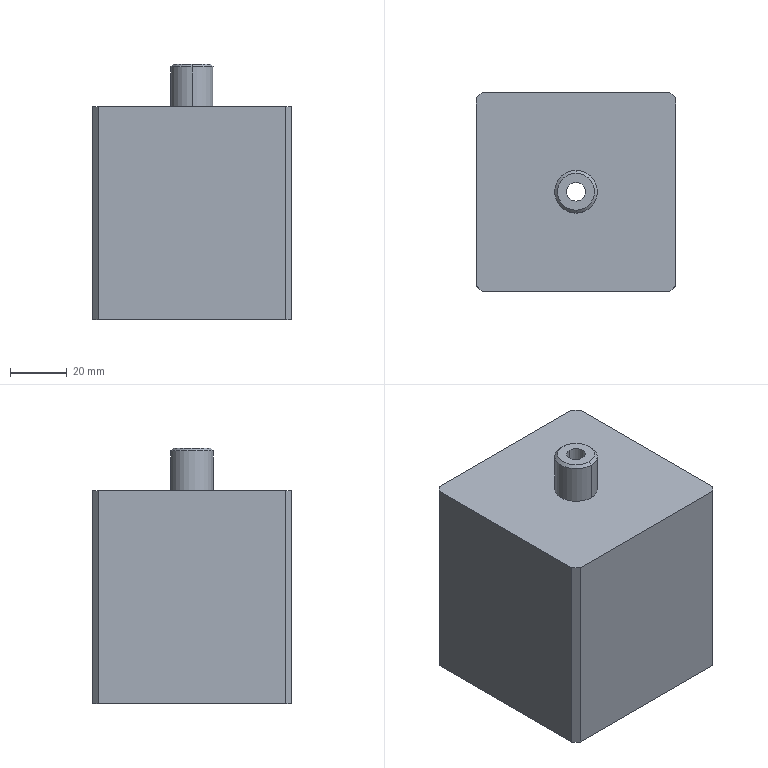NC program | NX | posted with a generic post | part box 70 x 70 x 90 mm
Lines 1716 to 2643 of 2643:
(FLOOR_WALL_1 , TOOL : D10)
N3406 T04 M6
N3408 G54
N3410 G17 G0 G90 X-41.5 Y3.262 S7500 M3
N3412 G43 Z30. H4
N3414 Z0.51
N3416 G94 G1 Z-0.99 F1000.
N3418 X-35.5 Y6.726
N3420 G3 X-35. Y7.592 R1.
N3422 G1 Y33. F2500.
N3424 X-33. Y35.
N3426 X33.
N3428 X35. Y33.
N3430 Y-33.
N3432 X33. Y-35.
N3434 X-33.
N3436 X-35. Y-33.
N3438 Y7.592
N3440 X-28.
N3442 Y28.
N3444 X28.
N3446 Y-28.
N3448 X-28.
N3450 Y7.592
N3452 X-21.
N3454 Y21.
N3456 X21.
N3458 Y1.184
N3460 X14.
N3462 G3 X1.184 Y14. R14.05
N3464 G1 X14.
N3466 Y1.184
N3468 X21.
N3470 Y-21.
N3472 X1.184
N3474 Y-14.
N3476 G3 X14. Y-1.184 R14.05
N3478 G1 Y-14.
N3480 X1.184
N3482 Y-21.
N3484 X-21.
N3486 Y-1.184
N3488 X-14.
N3490 G3 X-1.184 Y-14. R14.05
N3492 G1 X-14.
N3494 Y-1.184
N3496 X-21.
N3498 Y7.592
N3500 X-14.
N3502 Y14.
N3504 X-1.184
N3506 G3 X-14. Y1.184 R14.05
N3508 G1 X-12.605 Y1.066
N3510 G2 X1.066 Y12.605 R12.65
N3512 X-12.605 Y1.066 R-12.65
N3514 G1 X-14. Y1.184
N3516 Y7.592
N3518 G3 X-14.5 Y8.458 R1.
N3520 G1 Z0.51
N3522 G0 X-41.5 Y3.262 Z-0.48
N3524 G1 Z-1.98 F1000.
N3526 X-35.5 Y6.726
N3528 G3 X-35. Y7.592 R1.
N3530 G1 Y33. F2500.
N3532 X-33. Y35.
N3534 X33.
N3536 X35. Y33.
N3538 Y-33.
N3540 X33. Y-35.
N3542 X-33.
N3544 X-35. Y-33.
N3546 Y7.592
N3548 X-28.
N3550 Y28.
N3552 X28.
N3554 Y-28.
N3556 X-28.
N3558 Y7.592
N3560 X-21.
N3562 Y21.
N3564 X21.
N3566 Y1.184
N3568 X14.
N3570 G3 X1.184 Y14. R14.05
N3572 G1 X14.
N3574 Y1.184
N3576 X21.
N3578 Y-21.
N3580 X1.184
N3582 Y-14.
N3584 G3 X14. Y-1.184 R14.05
N3586 G1 Y-14.
N3588 X1.184
N3590 Y-21.
N3592 X-21.
N3594 Y-1.184
N3596 X-14.
N3598 G3 X-1.184 Y-14. R14.05
N3600 G1 X-14.
N3602 Y-1.184
N3604 X-21.
N3606 Y7.592
N3608 X-14.
N3610 Y14.
N3612 X-1.184
N3614 G3 X-14. Y1.184 R14.05
N3616 G1 X-12.605 Y1.066
N3618 G2 X1.066 Y12.605 R12.65
N3620 X-12.605 Y1.066 R-12.65
N3622 G1 X-14. Y1.184
N3624 Y7.592
N3626 G3 X-14.5 Y8.458 R1.
N3628 G1 Z-0.48
N3630 G0 X-41.5 Y3.262 Z-1.47
N3632 G1 Z-2.97 F1000.
N3634 X-35.5 Y6.726
N3636 G3 X-35. Y7.592 R1.
N3638 G1 Y33. F2500.
N3640 X-33. Y35.
N3642 X33.
N3644 X35. Y33.
N3646 Y-33.
N3648 X33. Y-35.
N3650 X-33.
N3652 X-35. Y-33.
N3654 Y7.592
N3656 X-28.
N3658 Y28.
N3660 X28.
N3662 Y-28.
N3664 X-28.
N3666 Y7.592
N3668 X-21.
N3670 Y21.
N3672 X21.
N3674 Y1.184
N3676 X14.
N3678 G3 X1.184 Y14. R14.05
N3680 G1 X14.
N3682 Y1.184
N3684 X21.
N3686 Y-21.
N3688 X1.184
N3690 Y-14.
N3692 G3 X14. Y-1.184 R14.05
N3694 G1 Y-14.
N3696 X1.184
N3698 Y-21.
N3700 X-21.
N3702 Y-1.184
N3704 X-14.
N3706 G3 X-1.184 Y-14. R14.05
N3708 G1 X-14.
N3710 Y-1.184
N3712 X-21.
N3714 Y7.592
N3716 X-14.
N3718 Y14.
N3720 X-1.184
N3722 G3 X-14. Y1.184 R14.05
N3724 G1 X-12.605 Y1.066
N3726 G2 X1.066 Y12.605 R12.65
N3728 X-12.605 Y1.066 R-12.65
N3730 G1 X-14. Y1.184
N3732 Y7.592
N3734 G3 X-14.5 Y8.458 R1.
N3736 G1 Z-1.47
N3738 G0 X-41.5 Y3.262 Z-2.46
N3740 G1 Z-3.96 F1000.
N3742 X-35.5 Y6.726
N3744 G3 X-35. Y7.592 R1.
N3746 G1 Y33. F2500.
N3748 X-33. Y35.
N3750 X33.
N3752 X35. Y33.
N3754 Y-33.
N3756 X33. Y-35.
N3758 X-33.
N3760 X-35. Y-33.
N3762 Y7.592
N3764 X-28.
N3766 Y28.
N3768 X28.
N3770 Y-28.
N3772 X-28.
N3774 Y7.592
N3776 X-21.
N3778 Y21.
N3780 X21.
N3782 Y1.184
N3784 X14.
N3786 G3 X1.184 Y14. R14.05
N3788 G1 X14.
N3790 Y1.184
N3792 X21.
N3794 Y-21.
N3796 X1.184
N3798 Y-14.
N3800 G3 X14. Y-1.184 R14.05
N3802 G1 Y-14.
N3804 X1.184
N3806 Y-21.
N3808 X-21.
N3810 Y-1.184
N3812 X-14.
N3814 G3 X-1.184 Y-14. R14.05
N3816 G1 X-14.
N3818 Y-1.184
N3820 X-21.
N3822 Y7.592
N3824 X-14.
N3826 Y14.
N3828 X-1.184
N3830 G3 X-14. Y1.184 R14.05
N3832 G1 X-12.605 Y1.066
N3834 G2 X1.066 Y12.605 R12.65
N3836 X-12.605 Y1.066 R-12.65
N3838 G1 X-14. Y1.184
N3840 Y7.592
N3842 G3 X-14.5 Y8.458 R1.
N3844 G1 Z-2.46
N3846 G0 X-41.5 Y3.262 Z-3.45
N3848 G1 Z-4.95 F1000.
N3850 X-35.5 Y6.726
N3852 G3 X-35. Y7.592 R1.
N3854 G1 Y33. F2500.
N3856 X-33. Y35.
N3858 X33.
N3860 X35. Y33.
N3862 Y-33.
N3864 X33. Y-35.
N3866 X-33.
N3868 X-35. Y-33.
N3870 Y7.592
N3872 X-28.
N3874 Y28.
N3876 X28.
N3878 Y-28.
N3880 X-28.
N3882 Y7.592
N3884 X-21.
N3886 Y21.
N3888 X21.
N3890 Y1.184
N3892 X14.
N3894 G3 X1.184 Y14. R14.05
N3896 G1 X14.
N3898 Y1.184
N3900 X21.
N3902 Y-21.
N3904 X1.184
N3906 Y-14.
N3908 G3 X14. Y-1.184 R14.05
N3910 G1 Y-14.
N3912 X1.184
N3914 Y-21.
N3916 X-21.
N3918 Y-1.184
N3920 X-14.
N3922 G3 X-1.184 Y-14. R14.05
N3924 G1 X-14.
N3926 Y-1.184
N3928 X-21.
N3930 Y7.592
N3932 X-14.
N3934 Y14.
N3936 X-1.184
N3938 G3 X-14. Y1.184 R14.05
N3940 G1 X-12.605 Y1.066
N3942 G2 X1.066 Y12.605 R12.65
N3944 X-12.605 Y1.066 R-12.65
N3946 G1 X-14. Y1.184
N3948 Y7.592
N3950 G3 X-14.5 Y8.458 R1.
N3952 G1 Z-3.45
N3954 G0 X-41.5 Y3.262 Z-4.44
N3956 G1 Z-5.94 F1000.
N3958 X-35.5 Y6.726
N3960 G3 X-35. Y7.592 R1.
N3962 G1 Y33. F2500.
N3964 X-33. Y35.
N3966 X33.
N3968 X35. Y33.
N3970 Y-33.
N3972 X33. Y-35.
N3974 X-33.
N3976 X-35. Y-33.
N3978 Y7.592
N3980 X-28.
N3982 Y28.
N3984 X28.
N3986 Y-28.
N3988 X-28.
N3990 Y7.592
N3992 X-21.
N3994 Y21.
N3996 X21.
N3998 Y1.184
N4000 X14.
N4002 G3 X1.184 Y14. R14.05
N4004 G1 X14.
N4006 Y1.184
N4008 X21.
N4010 Y-21.
N4012 X1.184
N4014 Y-14.
N4016 G3 X14. Y-1.184 R14.05
N4018 G1 Y-14.
N4020 X1.184
N4022 Y-21.
N4024 X-21.
N4026 Y-1.184
N4028 X-14.
N4030 G3 X-1.184 Y-14. R14.05
N4032 G1 X-14.
N4034 Y-1.184
N4036 X-21.
N4038 Y7.592
N4040 X-14.
N4042 Y14.
N4044 X-1.184
N4046 G3 X-14. Y1.184 R14.05
N4048 G1 X-12.605 Y1.066
N4050 G2 X1.066 Y12.605 R12.65
N4052 X-12.605 Y1.066 R-12.65
N4054 G1 X-14. Y1.184
N4056 Y7.592
N4058 G3 X-14.5 Y8.458 R1.
N4060 G1 Z-4.44
N4062 G0 X-41.5 Y3.262 Z-5.43
N4064 G1 Z-6.93 F1000.
N4066 X-35.5 Y6.726
N4068 G3 X-35. Y7.592 R1.
N4070 G1 Y33. F2500.
N4072 X-33. Y35.
N4074 X33.
N4076 X35. Y33.
N4078 Y-33.
N4080 X33. Y-35.
N4082 X-33.
N4084 X-35. Y-33.
N4086 Y7.592
N4088 X-28.
N4090 Y28.
N4092 X28.
N4094 Y-28.
N4096 X-28.
N4098 Y7.592
N4100 X-21.
N4102 Y21.
N4104 X21.
N4106 Y1.184
N4108 X14.
N4110 G3 X1.184 Y14. R14.05
N4112 G1 X14.
N4114 Y1.184
N4116 X21.
N4118 Y-21.
N4120 X1.184
N4122 Y-14.
N4124 G3 X14. Y-1.184 R14.05
N4126 G1 Y-14.
N4128 X1.184
N4130 Y-21.
N4132 X-21.
N4134 Y-1.184
N4136 X-14.
N4138 G3 X-1.184 Y-14. R14.05
N4140 G1 X-14.
N4142 Y-1.184
N4144 X-21.
N4146 Y7.592
N4148 X-14.
N4150 Y14.
N4152 X-1.184
N4154 G3 X-14. Y1.184 R14.05
N4156 G1 X-12.605 Y1.066
N4158 G2 X1.066 Y12.605 R12.65
N4160 X-12.605 Y1.066 R-12.65
N4162 G1 X-14. Y1.184
N4164 Y7.592
N4166 G3 X-14.5 Y8.458 R1.
N4168 G1 Z-5.43
N4170 G0 X-41.5 Y3.262 Z-6.42
N4172 G1 Z-7.92 F1000.
N4174 X-35.5 Y6.726
N4176 G3 X-35. Y7.592 R1.
N4178 G1 Y33. F2500.
N4180 X-33. Y35.
N4182 X33.
N4184 X35. Y33.
N4186 Y-33.
N4188 X33. Y-35.
N4190 X-33.
N4192 X-35. Y-33.
N4194 Y7.592
N4196 X-28.
N4198 Y28.
N4200 X28.
N4202 Y-28.
N4204 X-28.
N4206 Y7.592
N4208 X-21.
N4210 Y21.
N4212 X21.
N4214 Y1.184
N4216 X14.
N4218 G3 X1.184 Y14. R14.05
N4220 G1 X14.
N4222 Y1.184
N4224 X21.
N4226 Y-21.
N4228 X1.184
N4230 Y-14.
N4232 G3 X14. Y-1.184 R14.05
N4234 G1 Y-14.
N4236 X1.184
N4238 Y-21.
N4240 X-21.
N4242 Y-1.184
N4244 X-14.
N4246 G3 X-1.184 Y-14. R14.05
N4248 G1 X-14.
N4250 Y-1.184
N4252 X-21.
N4254 Y7.592
N4256 X-14.
N4258 Y14.
N4260 X-1.184
N4262 G3 X-14. Y1.184 R14.05
N4264 G1 X-12.605 Y1.066
N4266 G2 X1.066 Y12.605 R12.65
N4268 X-12.605 Y1.066 R-12.65
N4270 G1 X-14. Y1.184
N4272 Y7.592
N4274 G3 X-14.5 Y8.458 R1.
N4276 G1 Z-6.42
N4278 G0 X-41.5 Y3.262 Z-7.41
N4280 G1 Z-8.91 F1000.
N4282 X-35.5 Y6.726
N4284 G3 X-35. Y7.592 R1.
N4286 G1 Y33. F2500.
N4288 X-33. Y35.
N4290 X33.
N4292 X35. Y33.
N4294 Y-33.
N4296 X33. Y-35.
N4298 X-33.
N4300 X-35. Y-33.
N4302 Y7.592
N4304 X-28.
N4306 Y28.
N4308 X28.
N4310 Y-28.
N4312 X-28.
N4314 Y7.592
N4316 X-21.
N4318 Y21.
N4320 X21.
N4322 Y1.184
N4324 X14.
N4326 G3 X1.184 Y14. R14.05
N4328 G1 X14.
N4330 Y1.184
N4332 X21.
N4334 Y-21.
N4336 X1.184
N4338 Y-14.
N4340 G3 X14. Y-1.184 R14.05
N4342 G1 Y-14.
N4344 X1.184
N4346 Y-21.
N4348 X-21.
N4350 Y-1.184
N4352 X-14.
N4354 G3 X-1.184 Y-14. R14.05
N4356 G1 X-14.
N4358 Y-1.184
N4360 X-21.
N4362 Y7.592
N4364 X-14.
N4366 Y14.
N4368 X-1.184
N4370 G3 X-14. Y1.184 R14.05
N4372 G1 X-12.605 Y1.066
N4374 G2 X1.066 Y12.605 R12.65
N4376 X-12.605 Y1.066 R-12.65
N4378 G1 X-14. Y1.184
N4380 Y7.592
N4382 G3 X-14.5 Y8.458 R1.
N4384 G1 Z-7.41
N4386 G0 X-41.5 Y3.262 Z-8.4
N4388 G1 Z-9.9 F1000.
N4390 X-35.5 Y6.726
N4392 G3 X-35. Y7.592 R1.
N4394 G1 Y33. F2500.
N4396 X-33. Y35.
N4398 X33.
N4400 X35. Y33.
N4402 Y-33.
N4404 X33. Y-35.
N4406 X-33.
N4408 X-35. Y-33.
N4410 Y7.592
N4412 X-28.
N4414 Y28.
N4416 X28.
N4418 Y-28.
N4420 X-28.
N4422 Y7.592
N4424 X-21.
N4426 Y21.
N4428 X21.
N4430 Y1.184
N4432 X14.
N4434 G3 X1.184 Y14. R14.05
N4436 G1 X14.
N4438 Y1.184
N4440 X21.
N4442 Y-21.
N4444 X1.184
N4446 Y-14.
N4448 G3 X14. Y-1.184 R14.05
N4450 G1 Y-14.
N4452 X1.184
N4454 Y-21.
N4456 X-21.
N4458 Y-1.184
N4460 X-14.
N4462 G3 X-1.184 Y-14. R14.05
N4464 G1 X-14.
N4466 Y-1.184
N4468 X-21.
N4470 Y7.592
N4472 X-14.
N4474 Y14.
N4476 X-1.184
N4478 G3 X-14. Y1.184 R14.05
N4480 G1 X-12.605 Y1.066
N4482 G2 X1.066 Y12.605 R12.65
N4484 X-12.605 Y1.066 R-12.65
N4486 G1 X-14. Y1.184
N4488 Y7.592
N4490 G3 X-14.5 Y8.458 R1.
N4492 G1 Z-8.4
N4494 G0 X-41.5 Y3.262 Z-9.39
N4496 G1 Z-10.89 F1000.
N4498 X-35.5 Y6.726
N4500 G3 X-35. Y7.592 R1.
N4502 G1 Y33. F2500.
N4504 X-33. Y35.
N4506 X33.
N4508 X35. Y33.
N4510 Y-33.
N4512 X33. Y-35.
N4514 X-33.
N4516 X-35. Y-33.
N4518 Y7.592
N4520 X-28.
N4522 Y28.
N4524 X28.
N4526 Y-28.
N4528 X-28.
N4530 Y7.592
N4532 X-21.
N4534 Y21.
N4536 X21.
N4538 Y1.184
N4540 X14.
N4542 G3 X1.184 Y14. R14.05
N4544 G1 X14.
N4546 Y1.184
N4548 X21.
N4550 Y-21.
N4552 X1.184
N4554 Y-14.
N4556 G3 X14. Y-1.184 R14.05
N4558 G1 Y-14.
N4560 X1.184
N4562 Y-21.
N4564 X-21.
N4566 Y-1.184
N4568 X-14.
N4570 G3 X-1.184 Y-14. R14.05
N4572 G1 X-14.
N4574 Y-1.184
N4576 X-21.
N4578 Y7.592
N4580 X-14.
N4582 Y14.
N4584 X-1.184
N4586 G3 X-14. Y1.184 R14.05
N4588 G1 X-12.605 Y1.066
N4590 G2 X1.066 Y12.605 R12.65
N4592 X-12.605 Y1.066 R-12.65
N4594 G1 X-14. Y1.184
N4596 Y7.592
N4598 G3 X-14.5 Y8.458 R1.
N4600 G1 Z-9.39
N4602 G0 X-41.5 Y3.262 Z-10.38
N4604 G1 Z-11.88 F1000.
N4606 X-35.5 Y6.726
N4608 G3 X-35. Y7.592 R1.
N4610 G1 Y33. F2500.
N4612 X-33. Y35.
N4614 X33.
N4616 X35. Y33.
N4618 Y-33.
N4620 X33. Y-35.
N4622 X-33.
N4624 X-35. Y-33.
N4626 Y7.592
N4628 X-28.
N4630 Y28.
N4632 X28.
N4634 Y-28.
N4636 X-28.
N4638 Y7.592
N4640 X-21.
N4642 Y21.
N4644 X21.
N4646 Y1.184
N4648 X14.
N4650 G3 X1.184 Y14. R14.05
N4652 G1 X14.
N4654 Y1.184
N4656 X21.
N4658 Y-21.
N4660 X1.184
N4662 Y-14.
N4664 G3 X14. Y-1.184 R14.05
N4666 G1 Y-14.
N4668 X1.184
N4670 Y-21.
N4672 X-21.
N4674 Y-1.184
N4676 X-14.
N4678 G3 X-1.184 Y-14. R14.05
N4680 G1 X-14.
N4682 Y-1.184
N4684 X-21.
N4686 Y7.592
N4688 X-14.
N4690 Y14.
N4692 X-1.184
N4694 G3 X-14. Y1.184 R14.05
N4696 G1 X-12.605 Y1.066
N4698 G2 X1.066 Y12.605 R12.65
N4700 X-12.605 Y1.066 R-12.65
N4702 G1 X-14. Y1.184
N4704 Y7.592
N4706 G3 X-14.5 Y8.458 R1.
N4708 G1 Z-10.38
N4710 G0 X-41.5 Y3.262 Z-11.37
N4712 G1 Z-12.87 F1000.
N4714 X-35.5 Y6.726
N4716 G3 X-35. Y7.592 R1.
N4718 G1 Y33. F2500.
N4720 X-33. Y35.
N4722 X33.
N4724 X35. Y33.
N4726 Y-33.
N4728 X33. Y-35.
N4730 X-33.
N4732 X-35. Y-33.
N4734 Y7.592
N4736 X-28.
N4738 Y28.
N4740 X28.
N4742 Y-28.
N4744 X-28.
N4746 Y7.592
N4748 X-21.
N4750 Y21.
N4752 X21.
N4754 Y1.184
N4756 X14.
N4758 G3 X1.184 Y14. R14.05
N4760 G1 X14.
N4762 Y1.184
N4764 X21.
N4766 Y-21.
N4768 X1.184
N4770 Y-14.
N4772 G3 X14. Y-1.184 R14.05
N4774 G1 Y-14.
N4776 X1.184
N4778 Y-21.
N4780 X-21.
N4782 Y-1.184
N4784 X-14.
N4786 G3 X-1.184 Y-14. R14.05
N4788 G1 X-14.
N4790 Y-1.184
N4792 X-21.
N4794 Y7.592
N4796 X-14.
N4798 Y14.
N4800 X-1.184
N4802 G3 X-14. Y1.184 R14.05
N4804 G1 X-12.605 Y1.066
N4806 G2 X1.066 Y12.605 R12.65
N4808 X-12.605 Y1.066 R-12.65
N4810 G1 X-14. Y1.184
N4812 Y7.592
N4814 G3 X-14.5 Y8.458 R1.
N4816 G1 Z-11.37
N4818 G0 X-41.5 Y3.262 Z-12.36
N4820 G1 Z-13.86 F1000.
N4822 X-35.5 Y6.726
N4824 G3 X-35. Y7.592 R1.
N4826 G1 Y33. F2500.
N4828 X-33. Y35.
N4830 X33.
N4832 X35. Y33.
N4834 Y-33.
N4836 X33. Y-35.
N4838 X-33.
N4840 X-35. Y-33.
N4842 Y7.592
N4844 X-28.
N4846 Y28.
N4848 X28.
N4850 Y-28.
N4852 X-28.
N4854 Y7.592
N4856 X-21.
N4858 Y21.
N4860 X21.
N4862 Y1.184
N4864 X14.
N4866 G3 X1.184 Y14. R14.05
N4868 G1 X14.
N4870 Y1.184
N4872 X21.
N4874 Y-21.
N4876 X1.184
N4878 Y-14.
N4880 G3 X14. Y-1.184 R14.05
N4882 G1 Y-14.
N4884 X1.184
N4886 Y-21.
N4888 X-21.
N4890 Y-1.184
N4892 X-14.
N4894 G3 X-1.184 Y-14. R14.05
N4896 G1 X-14.
N4898 Y-1.184
N4900 X-21.
N4902 Y7.592
N4904 X-14.
N4906 Y14.
N4908 X-1.184
N4910 G3 X-14. Y1.184 R14.05
N4912 G1 X-12.605 Y1.066
N4914 G2 X1.066 Y12.605 R12.65
N4916 X-12.605 Y1.066 R-12.65
N4918 G1 X-14. Y1.184
N4920 Y7.592
N4922 G3 X-14.5 Y8.458 R1.
N4924 G1 Z-12.36
N4926 G0 X-41.5 Y3.262 Z-13.35
N4928 G1 Z-14.85 F1000.
N4930 X-35.5 Y6.726
N4932 G3 X-35. Y7.592 R1.
N4934 G1 Y33. F2500.
N4936 X-33. Y35.
N4938 X33.
N4940 X35. Y33.
N4942 Y-33.
N4944 X33. Y-35.
N4946 X-33.
N4948 X-35. Y-33.
N4950 Y7.592
N4952 X-28.
N4954 Y28.
N4956 X28.
N4958 Y-28.
N4960 X-28.
N4962 Y7.592
N4964 X-21.
N4966 Y21.
N4968 X21.
N4970 Y1.184
N4972 X14.
N4974 G3 X1.184 Y14. R14.05
N4976 G1 X14.
N4978 Y1.184
N4980 X21.
N4982 Y-21.
N4984 X1.184
N4986 Y-14.
N4988 G3 X14. Y-1.184 R14.05
N4990 G1 Y-14.
N4992 X1.184
N4994 Y-21.
N4996 X-21.
N4998 Y-1.184
N5000 X-14.
N5002 G3 X-1.184 Y-14. R14.05
N5004 G1 X-14.
N5006 Y-1.184
N5008 X-21.
N5010 Y7.592
N5012 X-14.
N5014 Y14.
N5016 X-1.184
N5018 G3 X-14. Y1.184 R14.05
N5020 G1 X-12.605 Y1.066
N5022 G2 X1.066 Y12.605 R12.65
N5024 X-12.605 Y1.066 R-12.65
N5026 G1 X-14. Y1.184
N5028 Y7.592
N5030 G3 X-14.5 Y8.458 R1.
N5032 G1 Z-13.35
N5034 G0 Z30.
(FLOOR_WALL_1_COPY , TOOL : D10)
N5036 X-41.165 Y36.015
N5038 Z-13.5
N5040 G1 Z-15. F1000.
N5042 X-40.866 Y35.497
N5044 G3 X-40. Y34.997 R1.
N5046 G1 X40.
N5048 Y28.397
N5050 X-40.
N5052 Y21.798
N5054 X40.
N5056 Y15.198
N5058 X-40.
N5060 Y8.598
N5062 X-9.75
N5064 G3 X-12.845 Y1.999 R13.
N5066 G1 X-40.
N5068 Y-4.601
N5070 X-12.158
N5072 G3 X-6.598 Y-11.201 R13.
N5074 G1 X-40.
N5076 G2 X-40.866 Y-10.701 R1.
N5078 G1 X-41.5 Y-9.603
N5080 Z-13.5
N5082 G0 Z-11.
N5084 G1 X-9.75 Y8.598 F8000.
N5086 G0 Z-13.5
N5088 G1 Z-15. F1000.
N5090 G2 X9.75 Y8.598 R13.
N5092 G1 X40.
N5094 Y1.999
N5096 X12.845
N5098 G2 X12.158 Y-4.601 R13.
N5100 G1 X40.
N5102 Y-11.201
N5104 X6.598
N5106 Z-13.5
N5108 G0 Z30.
N5110 X-41.5 Y-16.203
N5112 Z-13.5
N5114 G1 Z-15.
N5116 X-40.866 Y-17.301
N5118 G3 X-40. Y-17.801 R1.
N5120 G1 X40.
N5122 Y-24.4
N5124 X-40.
N5126 Y-31.
N5128 X40.
N5130 G3 X40.866 Y-30.5 R1.
N5132 G1 X41.5 Y-29.402
N5134 Z-13.5
N5136 G0 Z-11.
N5138 G1 X14.403 Y1.676 F8000.
N5140 G0 Z-13.5
N5142 G1 Z-15. F1000.
N5144 X13. Y0.866
N5146 G3 X12.5 Y0. R1.
N5148 G2 X0. Y-12.5 R12.5
N5150 X12.5 Y0. R-12.5
N5152 G3 X13. Y-0.866 R1.
N5154 G1 X14.403 Y-1.676
N5156 Z-13.5
N5158 G0 Z30.
N5160 M5
(PLANAR_MILL , TOOL : D8A45)
N5162 T06 M6
N5164 G54
N5166 G17 G0 G90 X0. Y-12. S7500 M3
N5168 G43 Z30. H6
N5170 Z1.5
N5172 G94 G1 Z-1.5 F1250.
N5174 Y-8.
N5176 G2 X-8. Y0. R8.
N5178 X0. Y-8. R-8.
N5180 G1 Y-12.
N5182 Z1.5
N5184 G0 Z30.
(PLANAR_MILL_COPY , TOOL : D8A45)
N5186 X-40.3 Y0.
N5188 Z-13.5
N5190 G1 Z-16.5
N5192 X-36.3
N5194 Y33.
N5196 G2 X-35.919 Y33.919 R1.3
N5198 G1 X-33.919 Y35.919
N5200 G2 X-33. Y36.3 R1.3
N5202 G1 X33.
N5204 G2 X33.919 Y35.919 R1.3
N5206 G1 X35.919 Y33.919
N5208 G2 X36.3 Y33. R1.3
N5210 G1 Y-33.
N5212 G2 X35.919 Y-33.919 R1.3
N5214 G1 X33.919 Y-35.919
N5216 G2 X33. Y-36.3 R1.3
N5218 G1 X-33.
N5220 G2 X-33.919 Y-35.919 R1.3
N5222 G1 X-35.919 Y-33.919
N5224 G2 X-36.3 Y-33. R1.3
N5226 G1 Y0.
N5228 X-40.3
N5230 Z-13.5
N5232 G0 Z30.
N5234 M5
N5236 M2